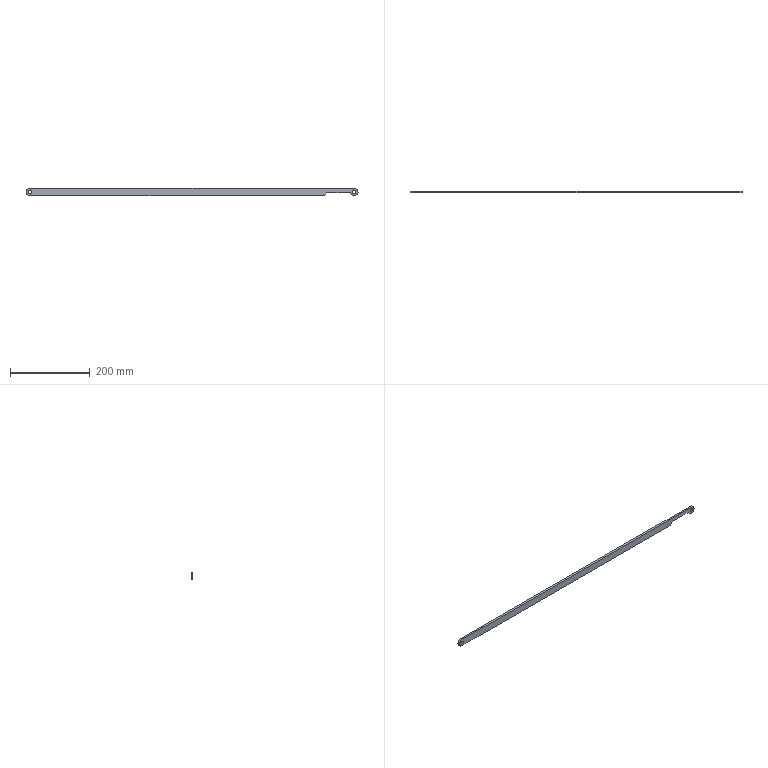Part | NX | features BREP 1 | 1 solid | 16 faces | box 833.12 x 4.763 x 19.05 mm | volume 72213 mm3 | cylinder 10 | plane 6 | commonest cylinder face diameters 8.382 x4 6.35 x3 19.05 x3
STEP:
#1=CARTESIAN_POINT('',(329.52,0.,-9.525));
#2=VERTEX_POINT('',#1);
#3=CARTESIAN_POINT('',(-407.035,0.,-9.525));
#4=VERTEX_POINT('',#3);
#5=CARTESIAN_POINT('',(329.52,0.,-9.525));
#6=DIRECTION('',(-1.,0.,0.));
#7=VECTOR('',#6,1000.);
#8=LINE('',#5,#7);
#9=EDGE_CURVE('',#2,#4,#8,.T.);
#10=ORIENTED_EDGE('',*,*,#9,.T.);
#11=CARTESIAN_POINT('',(-407.035,0.,9.525));
#12=VERTEX_POINT('',#11);
#13=CARTESIAN_POINT('',(-407.035,0.,0.));
#14=DIRECTION('',(0.,1.,0.));
#15=DIRECTION('',(0.,0.,-1.));
#16=AXIS2_PLACEMENT_3D('',#13,#14,#15);
#17=CIRCLE('',#16,9.525);
#18=EDGE_CURVE('',#4,#12,#17,.T.);
#19=ORIENTED_EDGE('',*,*,#18,.T.);
#20=CARTESIAN_POINT('',(407.035,0.,9.525));
#21=VERTEX_POINT('',#20);
#22=CARTESIAN_POINT('',(-407.035,0.,9.525));
#23=DIRECTION('',(1.,0.,0.));
#24=VECTOR('',#23,1000.);
#25=LINE('',#22,#24);
#26=EDGE_CURVE('',#12,#21,#25,.T.);
#27=ORIENTED_EDGE('',*,*,#26,.T.);
#28=CARTESIAN_POINT('',(407.035,0.,-9.525));
#29=VERTEX_POINT('',#28);
#30=CARTESIAN_POINT('',(407.035,0.,0.));
#31=DIRECTION('',(0.,1.,0.));
#32=DIRECTION('',(0.,0.,1.));
#33=AXIS2_PLACEMENT_3D('',#30,#31,#32);
#34=CIRCLE('',#33,9.525);
#35=EDGE_CURVE('',#21,#29,#34,.T.);
#36=ORIENTED_EDGE('',*,*,#35,.T.);
#37=CARTESIAN_POINT('',(398.186,0.,-3.524));
#38=VERTEX_POINT('',#37);
#39=CARTESIAN_POINT('',(407.035,0.,0.));
#40=DIRECTION('',(0.,1.,0.));
#41=DIRECTION('',(0.000000045,0.,-1.));
#42=AXIS2_PLACEMENT_3D('',#39,#40,#41);
#43=CIRCLE('',#42,9.525);
#44=EDGE_CURVE('',#29,#38,#43,.T.);
#45=ORIENTED_EDGE('',*,*,#44,.T.);
#46=CARTESIAN_POINT('',(395.236,0.,-1.524));
#47=VERTEX_POINT('',#46);
#48=CARTESIAN_POINT('',(395.236,0.,-4.699));
#49=DIRECTION('',(0.,-1.,0.));
#50=DIRECTION('',(0.929,0.,0.37));
#51=AXIS2_PLACEMENT_3D('',#48,#49,#50);
#52=CIRCLE('',#51,3.175);
#53=EDGE_CURVE('',#38,#47,#52,.T.);
#54=ORIENTED_EDGE('',*,*,#53,.T.);
#55=CARTESIAN_POINT('',(340.151,0.,-1.524));
#56=VERTEX_POINT('',#55);
#57=CARTESIAN_POINT('',(395.236,0.,-1.524));
#58=DIRECTION('',(-1.,0.,0.));
#59=VECTOR('',#58,1000.);
#60=LINE('',#57,#59);
#61=EDGE_CURVE('',#47,#56,#60,.T.);
#62=ORIENTED_EDGE('',*,*,#61,.T.);
#63=CARTESIAN_POINT('',(337.906,0.,-2.454));
#64=VERTEX_POINT('',#63);
#65=CARTESIAN_POINT('',(340.151,0.,-4.699));
#66=DIRECTION('',(0.,-1.,0.));
#67=DIRECTION('',(0.,0.,1.));
#68=AXIS2_PLACEMENT_3D('',#65,#66,#67);
#69=CIRCLE('',#68,3.175);
#70=EDGE_CURVE('',#56,#64,#69,.T.);
#71=ORIENTED_EDGE('',*,*,#70,.T.);
#72=CARTESIAN_POINT('',(331.765,0.,-8.595));
#73=VERTEX_POINT('',#72);
#74=CARTESIAN_POINT('',(337.906,0.,-2.454));
#75=DIRECTION('',(-0.7071,0.,-0.7071));
#76=VECTOR('',#75,1000.);
#77=LINE('',#74,#76);
#78=EDGE_CURVE('',#64,#73,#77,.T.);
#79=ORIENTED_EDGE('',*,*,#78,.T.);
#80=CARTESIAN_POINT('',(329.52,0.,-6.35));
#81=DIRECTION('',(0.,1.,0.));
#82=DIRECTION('',(0.7071,0.,-0.7071));
#83=AXIS2_PLACEMENT_3D('',#80,#81,#82);
#84=CIRCLE('',#83,3.175);
#85=EDGE_CURVE('',#73,#2,#84,.T.);
#86=ORIENTED_EDGE('',*,*,#85,.T.);
#87=EDGE_LOOP('',(#10,#19,#27,#36,#45,#54,#62,#71,#79,#86));
#88=FACE_BOUND('',#87,.T.);
#89=CARTESIAN_POINT('',(-411.226,0.,0.));
#90=VERTEX_POINT('',#89);
#91=CARTESIAN_POINT('',(-402.844,0.,0.));
#92=VERTEX_POINT('',#91);
#93=CARTESIAN_POINT('',(-407.035,0.,0.));
#94=DIRECTION('',(0.,-1.,0.));
#95=DIRECTION('',(-1.,0.,0.));
#96=AXIS2_PLACEMENT_3D('',#93,#94,#95);
#97=CIRCLE('',#96,4.191);
#98=EDGE_CURVE('',#90,#92,#97,.T.);
#99=ORIENTED_EDGE('',*,*,#98,.T.);
#100=CARTESIAN_POINT('',(-407.035,0.,0.));
#101=DIRECTION('',(0.,-1.,0.));
#102=DIRECTION('',(1.,0.,0.));
#103=AXIS2_PLACEMENT_3D('',#100,#101,#102);
#104=CIRCLE('',#103,4.191);
#105=EDGE_CURVE('',#92,#90,#104,.T.);
#106=ORIENTED_EDGE('',*,*,#105,.T.);
#107=EDGE_LOOP('',(#99,#106));
#108=FACE_BOUND('',#107,.T.);
#109=CARTESIAN_POINT('',(402.844,0.,0.));
#110=VERTEX_POINT('',#109);
#111=CARTESIAN_POINT('',(411.226,0.,0.));
#112=VERTEX_POINT('',#111);
#113=CARTESIAN_POINT('',(407.035,0.,0.));
#114=DIRECTION('',(0.,-1.,0.));
#115=DIRECTION('',(-1.,0.,0.));
#116=AXIS2_PLACEMENT_3D('',#113,#114,#115);
#117=CIRCLE('',#116,4.191);
#118=EDGE_CURVE('',#110,#112,#117,.T.);
#119=ORIENTED_EDGE('',*,*,#118,.T.);
#120=CARTESIAN_POINT('',(407.035,0.,0.));
#121=DIRECTION('',(0.,-1.,0.));
#122=DIRECTION('',(1.,0.,0.));
#123=AXIS2_PLACEMENT_3D('',#120,#121,#122);
#124=CIRCLE('',#123,4.191);
#125=EDGE_CURVE('',#112,#110,#124,.T.);
#126=ORIENTED_EDGE('',*,*,#125,.T.);
#127=EDGE_LOOP('',(#119,#126));
#128=FACE_BOUND('',#127,.T.);
#129=CARTESIAN_POINT('',(0.,0.,0.));
#130=DIRECTION('',(0.,1.,0.));
#131=DIRECTION('',(1.,0.,0.));
#132=AXIS2_PLACEMENT_3D('',#129,#130,#131);
#133=PLANE('',#132);
#134=ADVANCED_FACE('',(#88,#108,#128),#133,.T.);
#135=CARTESIAN_POINT('',(411.226,-4.763,0.));
#136=VERTEX_POINT('',#135);
#137=CARTESIAN_POINT('',(411.226,0.,0.));
#138=DIRECTION('',(0.,-1.,0.));
#139=VECTOR('',#138,1000.);
#140=LINE('',#137,#139);
#141=EDGE_CURVE('',#136,#112,#140,.F.);
#142=ORIENTED_EDGE('',*,*,#141,.F.);
#143=CARTESIAN_POINT('',(402.844,-4.763,0.));
#144=VERTEX_POINT('',#143);
#145=CARTESIAN_POINT('',(407.035,-4.763,0.));
#146=DIRECTION('',(0.,-1.,0.));
#147=DIRECTION('',(1.,0.,0.));
#148=AXIS2_PLACEMENT_3D('',#145,#146,#147);
#149=CIRCLE('',#148,4.191);
#150=EDGE_CURVE('',#136,#144,#149,.T.);
#151=ORIENTED_EDGE('',*,*,#150,.T.);
#152=CARTESIAN_POINT('',(402.844,0.,0.));
#153=DIRECTION('',(0.,-1.,0.));
#154=VECTOR('',#153,1000.);
#155=LINE('',#152,#154);
#156=EDGE_CURVE('',#144,#110,#155,.F.);
#157=ORIENTED_EDGE('',*,*,#156,.T.);
#158=ORIENTED_EDGE('',*,*,#125,.F.);
#159=EDGE_LOOP('',(#142,#151,#157,#158));
#160=FACE_BOUND('',#159,.T.);
#161=CARTESIAN_POINT('',(407.035,0.,0.));
#162=DIRECTION('',(0.,-1.,0.));
#163=DIRECTION('',(1.,0.,0.));
#164=AXIS2_PLACEMENT_3D('',#161,#162,#163);
#165=CYLINDRICAL_SURFACE('',#164,4.191);
#166=ADVANCED_FACE('',(#160),#165,.F.);
#167=ORIENTED_EDGE('',*,*,#156,.F.);
#168=CARTESIAN_POINT('',(407.035,-4.763,0.));
#169=DIRECTION('',(0.,-1.,0.));
#170=DIRECTION('',(-1.,0.,0.));
#171=AXIS2_PLACEMENT_3D('',#168,#169,#170);
#172=CIRCLE('',#171,4.191);
#173=EDGE_CURVE('',#144,#136,#172,.T.);
#174=ORIENTED_EDGE('',*,*,#173,.T.);
#175=ORIENTED_EDGE('',*,*,#141,.T.);
#176=ORIENTED_EDGE('',*,*,#118,.F.);
#177=EDGE_LOOP('',(#167,#174,#175,#176));
#178=FACE_BOUND('',#177,.T.);
#179=CARTESIAN_POINT('',(407.035,0.,0.));
#180=DIRECTION('',(0.,-1.,0.));
#181=DIRECTION('',(1.,0.,0.));
#182=AXIS2_PLACEMENT_3D('',#179,#180,#181);
#183=CYLINDRICAL_SURFACE('',#182,4.191);
#184=ADVANCED_FACE('',(#178),#183,.F.);
#185=CARTESIAN_POINT('',(337.906,-4.763,-2.454));
#186=VERTEX_POINT('',#185);
#187=CARTESIAN_POINT('',(331.765,-4.763,-8.595));
#188=VERTEX_POINT('',#187);
#189=CARTESIAN_POINT('',(337.906,-4.763,-2.454));
#190=DIRECTION('',(-0.7071,0.,-0.7071));
#191=VECTOR('',#190,1000.);
#192=LINE('',#189,#191);
#193=EDGE_CURVE('',#186,#188,#192,.T.);
#194=ORIENTED_EDGE('',*,*,#193,.F.);
#195=CARTESIAN_POINT('',(340.151,-4.763,-1.524));
#196=VERTEX_POINT('',#195);
#197=CARTESIAN_POINT('',(340.151,-4.763,-4.699));
#198=DIRECTION('',(0.,1.,0.));
#199=DIRECTION('',(-0.7071,0.,0.7071));
#200=AXIS2_PLACEMENT_3D('',#197,#198,#199);
#201=CIRCLE('',#200,3.175);
#202=EDGE_CURVE('',#186,#196,#201,.T.);
#203=ORIENTED_EDGE('',*,*,#202,.T.);
#204=CARTESIAN_POINT('',(395.236,-4.763,-1.524));
#205=VERTEX_POINT('',#204);
#206=CARTESIAN_POINT('',(395.236,-4.763,-1.524));
#207=DIRECTION('',(-1.,0.,0.));
#208=VECTOR('',#207,1000.);
#209=LINE('',#206,#208);
#210=EDGE_CURVE('',#205,#196,#209,.T.);
#211=ORIENTED_EDGE('',*,*,#210,.F.);
#212=CARTESIAN_POINT('',(398.186,-4.763,-3.524));
#213=VERTEX_POINT('',#212);
#214=CARTESIAN_POINT('',(395.236,-4.763,-4.699));
#215=DIRECTION('',(0.,1.,0.));
#216=DIRECTION('',(0.,0.,1.));
#217=AXIS2_PLACEMENT_3D('',#214,#215,#216);
#218=CIRCLE('',#217,3.175);
#219=EDGE_CURVE('',#205,#213,#218,.T.);
#220=ORIENTED_EDGE('',*,*,#219,.T.);
#221=CARTESIAN_POINT('',(407.035,-4.763,-9.525));
#222=VERTEX_POINT('',#221);
#223=CARTESIAN_POINT('',(407.035,-4.763,0.));
#224=DIRECTION('',(0.,1.,0.));
#225=DIRECTION('',(0.000000045,0.,-1.));
#226=AXIS2_PLACEMENT_3D('',#223,#224,#225);
#227=CIRCLE('',#226,9.525);
#228=EDGE_CURVE('',#222,#213,#227,.T.);
#229=ORIENTED_EDGE('',*,*,#228,.F.);
#230=CARTESIAN_POINT('',(407.035,-4.763,9.525));
#231=VERTEX_POINT('',#230);
#232=CARTESIAN_POINT('',(407.035,-4.763,0.));
#233=DIRECTION('',(0.,1.,0.));
#234=DIRECTION('',(0.,0.,1.));
#235=AXIS2_PLACEMENT_3D('',#232,#233,#234);
#236=CIRCLE('',#235,9.525);
#237=EDGE_CURVE('',#231,#222,#236,.T.);
#238=ORIENTED_EDGE('',*,*,#237,.F.);
#239=CARTESIAN_POINT('',(-407.035,-4.763,9.525));
#240=VERTEX_POINT('',#239);
#241=CARTESIAN_POINT('',(-407.035,-4.763,9.525));
#242=DIRECTION('',(1.,0.,0.));
#243=VECTOR('',#242,1000.);
#244=LINE('',#241,#243);
#245=EDGE_CURVE('',#240,#231,#244,.T.);
#246=ORIENTED_EDGE('',*,*,#245,.F.);
#247=CARTESIAN_POINT('',(-407.035,-4.763,-9.525));
#248=VERTEX_POINT('',#247);
#249=CARTESIAN_POINT('',(-407.035,-4.763,0.));
#250=DIRECTION('',(0.,1.,0.));
#251=DIRECTION('',(0.,0.,-1.));
#252=AXIS2_PLACEMENT_3D('',#249,#250,#251);
#253=CIRCLE('',#252,9.525);
#254=EDGE_CURVE('',#248,#240,#253,.T.);
#255=ORIENTED_EDGE('',*,*,#254,.F.);
#256=CARTESIAN_POINT('',(329.52,-4.763,-9.525));
#257=VERTEX_POINT('',#256);
#258=CARTESIAN_POINT('',(329.52,-4.763,-9.525));
#259=DIRECTION('',(-1.,0.,0.));
#260=VECTOR('',#259,1000.);
#261=LINE('',#258,#260);
#262=EDGE_CURVE('',#257,#248,#261,.T.);
#263=ORIENTED_EDGE('',*,*,#262,.F.);
#264=CARTESIAN_POINT('',(329.52,-4.763,-6.35));
#265=DIRECTION('',(0.,-1.,0.));
#266=DIRECTION('',(0.,0.,-1.));
#267=AXIS2_PLACEMENT_3D('',#264,#265,#266);
#268=CIRCLE('',#267,3.175);
#269=EDGE_CURVE('',#257,#188,#268,.T.);
#270=ORIENTED_EDGE('',*,*,#269,.T.);
#271=EDGE_LOOP('',(#194,#203,#211,#220,#229,#238,#246,#255,#263,#270));
#272=FACE_BOUND('',#271,.T.);
#273=CARTESIAN_POINT('',(-411.226,-4.763,0.));
#274=VERTEX_POINT('',#273);
#275=CARTESIAN_POINT('',(-402.844,-4.763,0.));
#276=VERTEX_POINT('',#275);
#277=CARTESIAN_POINT('',(-407.035,-4.763,0.));
#278=DIRECTION('',(0.,-1.,0.));
#279=DIRECTION('',(-1.,0.,0.));
#280=AXIS2_PLACEMENT_3D('',#277,#278,#279);
#281=CIRCLE('',#280,4.191);
#282=EDGE_CURVE('',#274,#276,#281,.T.);
#283=ORIENTED_EDGE('',*,*,#282,.F.);
#284=CARTESIAN_POINT('',(-407.035,-4.763,0.));
#285=DIRECTION('',(0.,-1.,0.));
#286=DIRECTION('',(1.,0.,0.));
#287=AXIS2_PLACEMENT_3D('',#284,#285,#286);
#288=CIRCLE('',#287,4.191);
#289=EDGE_CURVE('',#276,#274,#288,.T.);
#290=ORIENTED_EDGE('',*,*,#289,.F.);
#291=EDGE_LOOP('',(#283,#290));
#292=FACE_BOUND('',#291,.T.);
#293=ORIENTED_EDGE('',*,*,#173,.F.);
#294=ORIENTED_EDGE('',*,*,#150,.F.);
#295=EDGE_LOOP('',(#293,#294));
#296=FACE_BOUND('',#295,.T.);
#297=CARTESIAN_POINT('',(0.,-4.763,0.));
#298=DIRECTION('',(0.,1.,0.));
#299=DIRECTION('',(1.,0.,0.));
#300=AXIS2_PLACEMENT_3D('',#297,#298,#299);
#301=PLANE('',#300);
#302=ADVANCED_FACE('',(#272,#292,#296),#301,.F.);
#303=CARTESIAN_POINT('',(-402.844,0.,0.));
#304=DIRECTION('',(0.,-1.,0.));
#305=VECTOR('',#304,1000.);
#306=LINE('',#303,#305);
#307=EDGE_CURVE('',#276,#92,#306,.F.);
#308=ORIENTED_EDGE('',*,*,#307,.F.);
#309=ORIENTED_EDGE('',*,*,#289,.T.);
#310=CARTESIAN_POINT('',(-411.226,0.,0.));
#311=DIRECTION('',(0.,-1.,0.));
#312=VECTOR('',#311,1000.);
#313=LINE('',#310,#312);
#314=EDGE_CURVE('',#274,#90,#313,.F.);
#315=ORIENTED_EDGE('',*,*,#314,.T.);
#316=ORIENTED_EDGE('',*,*,#105,.F.);
#317=EDGE_LOOP('',(#308,#309,#315,#316));
#318=FACE_BOUND('',#317,.T.);
#319=CARTESIAN_POINT('',(-407.035,0.,0.));
#320=DIRECTION('',(0.,-1.,0.));
#321=DIRECTION('',(1.,0.,0.));
#322=AXIS2_PLACEMENT_3D('',#319,#320,#321);
#323=CYLINDRICAL_SURFACE('',#322,4.191);
#324=ADVANCED_FACE('',(#318),#323,.F.);
#325=ORIENTED_EDGE('',*,*,#314,.F.);
#326=ORIENTED_EDGE('',*,*,#282,.T.);
#327=ORIENTED_EDGE('',*,*,#307,.T.);
#328=ORIENTED_EDGE('',*,*,#98,.F.);
#329=EDGE_LOOP('',(#325,#326,#327,#328));
#330=FACE_BOUND('',#329,.T.);
#331=CARTESIAN_POINT('',(-407.035,0.,0.));
#332=DIRECTION('',(0.,-1.,0.));
#333=DIRECTION('',(1.,0.,0.));
#334=AXIS2_PLACEMENT_3D('',#331,#332,#333);
#335=CYLINDRICAL_SURFACE('',#334,4.191);
#336=ADVANCED_FACE('',(#330),#335,.F.);
#337=ORIENTED_EDGE('',*,*,#269,.F.);
#338=CARTESIAN_POINT('',(329.52,-4.763,-9.525));
#339=DIRECTION('',(0.,1.,0.));
#340=VECTOR('',#339,1000.);
#341=LINE('',#338,#340);
#342=EDGE_CURVE('',#257,#2,#341,.T.);
#343=ORIENTED_EDGE('',*,*,#342,.T.);
#344=ORIENTED_EDGE('',*,*,#85,.F.);
#345=CARTESIAN_POINT('',(331.765,-4.763,-8.595));
#346=DIRECTION('',(0.,1.,0.));
#347=VECTOR('',#346,1000.);
#348=LINE('',#345,#347);
#349=EDGE_CURVE('',#188,#73,#348,.T.);
#350=ORIENTED_EDGE('',*,*,#349,.F.);
#351=EDGE_LOOP('',(#337,#343,#344,#350));
#352=FACE_BOUND('',#351,.T.);
#353=CARTESIAN_POINT('',(329.52,-5.988,-6.35));
#354=DIRECTION('',(0.,1.,0.));
#355=DIRECTION('',(0.7071,0.,-0.7071));
#356=AXIS2_PLACEMENT_3D('',#353,#354,#355);
#357=CYLINDRICAL_SURFACE('',#356,3.175);
#358=ADVANCED_FACE('',(#352),#357,.T.);
#359=ORIENTED_EDGE('',*,*,#78,.F.);
#360=CARTESIAN_POINT('',(337.906,0.,-2.454));
#361=DIRECTION('',(0.,-1.,0.));
#362=VECTOR('',#361,1000.);
#363=LINE('',#360,#362);
#364=EDGE_CURVE('',#64,#186,#363,.T.);
#365=ORIENTED_EDGE('',*,*,#364,.T.);
#366=ORIENTED_EDGE('',*,*,#193,.T.);
#367=ORIENTED_EDGE('',*,*,#349,.T.);
#368=EDGE_LOOP('',(#359,#365,#366,#367));
#369=FACE_BOUND('',#368,.T.);
#370=CARTESIAN_POINT('',(334.836,-2.381,-5.524));
#371=DIRECTION('',(0.7071,0.,-0.7071));
#372=DIRECTION('',(0.,-1.,0.));
#373=AXIS2_PLACEMENT_3D('',#370,#371,#372);
#374=PLANE('',#373);
#375=ADVANCED_FACE('',(#369),#374,.T.);
#376=ORIENTED_EDGE('',*,*,#202,.F.);
#377=ORIENTED_EDGE('',*,*,#364,.F.);
#378=ORIENTED_EDGE('',*,*,#70,.F.);
#379=CARTESIAN_POINT('',(340.151,0.,-1.524));
#380=DIRECTION('',(0.,-1.,0.));
#381=VECTOR('',#380,1000.);
#382=LINE('',#379,#381);
#383=EDGE_CURVE('',#56,#196,#382,.T.);
#384=ORIENTED_EDGE('',*,*,#383,.T.);
#385=EDGE_LOOP('',(#376,#377,#378,#384));
#386=FACE_BOUND('',#385,.T.);
#387=CARTESIAN_POINT('',(340.151,1.434,-4.699));
#388=DIRECTION('',(0.,-1.,0.));
#389=DIRECTION('',(0.,0.,1.));
#390=AXIS2_PLACEMENT_3D('',#387,#388,#389);
#391=CYLINDRICAL_SURFACE('',#390,3.175);
#392=ADVANCED_FACE('',(#386),#391,.F.);
#393=ORIENTED_EDGE('',*,*,#61,.F.);
#394=CARTESIAN_POINT('',(395.236,0.,-1.524));
#395=DIRECTION('',(0.,-1.,0.));
#396=VECTOR('',#395,1000.);
#397=LINE('',#394,#396);
#398=EDGE_CURVE('',#47,#205,#397,.T.);
#399=ORIENTED_EDGE('',*,*,#398,.T.);
#400=ORIENTED_EDGE('',*,*,#210,.T.);
#401=ORIENTED_EDGE('',*,*,#383,.F.);
#402=EDGE_LOOP('',(#393,#399,#400,#401));
#403=FACE_BOUND('',#402,.T.);
#404=CARTESIAN_POINT('',(368.234,-2.381,-1.524));
#405=DIRECTION('',(0.,0.,-1.));
#406=DIRECTION('',(0.,-1.,0.));
#407=AXIS2_PLACEMENT_3D('',#404,#405,#406);
#408=PLANE('',#407);
#409=ADVANCED_FACE('',(#403),#408,.T.);
#410=ORIENTED_EDGE('',*,*,#219,.F.);
#411=ORIENTED_EDGE('',*,*,#398,.F.);
#412=ORIENTED_EDGE('',*,*,#53,.F.);
#413=CARTESIAN_POINT('',(398.186,0.,-3.524));
#414=DIRECTION('',(0.,-1.,0.));
#415=VECTOR('',#414,1000.);
#416=LINE('',#413,#415);
#417=EDGE_CURVE('',#38,#213,#416,.T.);
#418=ORIENTED_EDGE('',*,*,#417,.T.);
#419=EDGE_LOOP('',(#410,#411,#412,#418));
#420=FACE_BOUND('',#419,.T.);
#421=CARTESIAN_POINT('',(395.236,1.434,-4.699));
#422=DIRECTION('',(0.,-1.,0.));
#423=DIRECTION('',(0.929,0.,0.37));
#424=AXIS2_PLACEMENT_3D('',#421,#422,#423);
#425=CYLINDRICAL_SURFACE('',#424,3.175);
#426=ADVANCED_FACE('',(#420),#425,.F.);
#427=ORIENTED_EDGE('',*,*,#44,.F.);
#428=CARTESIAN_POINT('',(407.035,0.,-9.525));
#429=DIRECTION('',(0.,-1.,0.));
#430=VECTOR('',#429,1000.);
#431=LINE('',#428,#430);
#432=EDGE_CURVE('',#29,#222,#431,.T.);
#433=ORIENTED_EDGE('',*,*,#432,.T.);
#434=ORIENTED_EDGE('',*,*,#228,.T.);
#435=ORIENTED_EDGE('',*,*,#417,.F.);
#436=EDGE_LOOP('',(#427,#433,#434,#435));
#437=FACE_BOUND('',#436,.T.);
#438=CARTESIAN_POINT('',(407.035,-2.381,0.));
#439=DIRECTION('',(0.,1.,0.));
#440=DIRECTION('',(0.000000102,0.,-1.));
#441=AXIS2_PLACEMENT_3D('',#438,#439,#440);
#442=CYLINDRICAL_SURFACE('',#441,9.525);
#443=ADVANCED_FACE('',(#437),#442,.T.);
#444=ORIENTED_EDGE('',*,*,#35,.F.);
#445=CARTESIAN_POINT('',(407.035,0.,9.525));
#446=DIRECTION('',(0.,-1.,0.));
#447=VECTOR('',#446,1000.);
#448=LINE('',#445,#447);
#449=EDGE_CURVE('',#21,#231,#448,.T.);
#450=ORIENTED_EDGE('',*,*,#449,.T.);
#451=ORIENTED_EDGE('',*,*,#237,.T.);
#452=ORIENTED_EDGE('',*,*,#432,.F.);
#453=EDGE_LOOP('',(#444,#450,#451,#452));
#454=FACE_BOUND('',#453,.T.);
#455=CARTESIAN_POINT('',(407.035,-2.381,0.));
#456=DIRECTION('',(0.,1.,0.));
#457=DIRECTION('',(0.,0.,1.));
#458=AXIS2_PLACEMENT_3D('',#455,#456,#457);
#459=CYLINDRICAL_SURFACE('',#458,9.525);
#460=ADVANCED_FACE('',(#454),#459,.T.);
#461=CARTESIAN_POINT('',(-407.035,0.,9.525));
#462=DIRECTION('',(0.,-1.,0.));
#463=VECTOR('',#462,1000.);
#464=LINE('',#461,#463);
#465=EDGE_CURVE('',#12,#240,#464,.T.);
#466=ORIENTED_EDGE('',*,*,#465,.T.);
#467=ORIENTED_EDGE('',*,*,#245,.T.);
#468=ORIENTED_EDGE('',*,*,#449,.F.);
#469=ORIENTED_EDGE('',*,*,#26,.F.);
#470=EDGE_LOOP('',(#466,#467,#468,#469));
#471=FACE_BOUND('',#470,.T.);
#472=CARTESIAN_POINT('',(0.,-2.381,9.525));
#473=DIRECTION('',(0.,0.,1.));
#474=DIRECTION('',(1.,0.,0.));
#475=AXIS2_PLACEMENT_3D('',#472,#473,#474);
#476=PLANE('',#475);
#477=ADVANCED_FACE('',(#471),#476,.T.);
#478=CARTESIAN_POINT('',(-407.035,0.,-9.525));
#479=DIRECTION('',(0.,-1.,0.));
#480=VECTOR('',#479,1000.);
#481=LINE('',#478,#480);
#482=EDGE_CURVE('',#4,#248,#481,.T.);
#483=ORIENTED_EDGE('',*,*,#482,.T.);
#484=ORIENTED_EDGE('',*,*,#254,.T.);
#485=ORIENTED_EDGE('',*,*,#465,.F.);
#486=ORIENTED_EDGE('',*,*,#18,.F.);
#487=EDGE_LOOP('',(#483,#484,#485,#486));
#488=FACE_BOUND('',#487,.T.);
#489=CARTESIAN_POINT('',(-407.035,-2.381,0.));
#490=DIRECTION('',(0.,1.,0.));
#491=DIRECTION('',(0.,0.,-1.));
#492=AXIS2_PLACEMENT_3D('',#489,#490,#491);
#493=CYLINDRICAL_SURFACE('',#492,9.525);
#494=ADVANCED_FACE('',(#488),#493,.T.);
#495=ORIENTED_EDGE('',*,*,#262,.T.);
#496=ORIENTED_EDGE('',*,*,#482,.F.);
#497=ORIENTED_EDGE('',*,*,#9,.F.);
#498=ORIENTED_EDGE('',*,*,#342,.F.);
#499=EDGE_LOOP('',(#495,#496,#497,#498));
#500=FACE_BOUND('',#499,.T.);
#501=CARTESIAN_POINT('',(0.,-2.381,-9.525));
#502=DIRECTION('',(0.,0.,-1.));
#503=DIRECTION('',(0.,-1.,0.));
#504=AXIS2_PLACEMENT_3D('',#501,#502,#503);
#505=PLANE('',#504);
#506=ADVANCED_FACE('',(#500),#505,.T.);
#507=CLOSED_SHELL('',(#134,#166,#184,#302,#324,#336,#358,#375,#392,#409,#426,#443,#460,#477,#494,#506));
#508=MANIFOLD_SOLID_BREP('',#507);
#509=(LENGTH_UNIT()NAMED_UNIT(*)SI_UNIT(.MILLI.,.METRE.));
#510=UNCERTAINTY_MEASURE_WITH_UNIT(LENGTH_MEASURE(0.00001),#509,'','');
#511=(NAMED_UNIT(*)PLANE_ANGLE_UNIT()SI_UNIT($,.RADIAN.));
#512=(NAMED_UNIT(*)SI_UNIT($,.STERADIAN.)SOLID_ANGLE_UNIT());
#513=(GEOMETRIC_REPRESENTATION_CONTEXT(3)GLOBAL_UNCERTAINTY_ASSIGNED_CONTEXT((#510))GLOBAL_UNIT_ASSIGNED_CONTEXT((#509,#511,#512))REPRESENTATION_CONTEXT('',''));
#514=ADVANCED_BREP_SHAPE_REPRESENTATION('',(#508),#513);